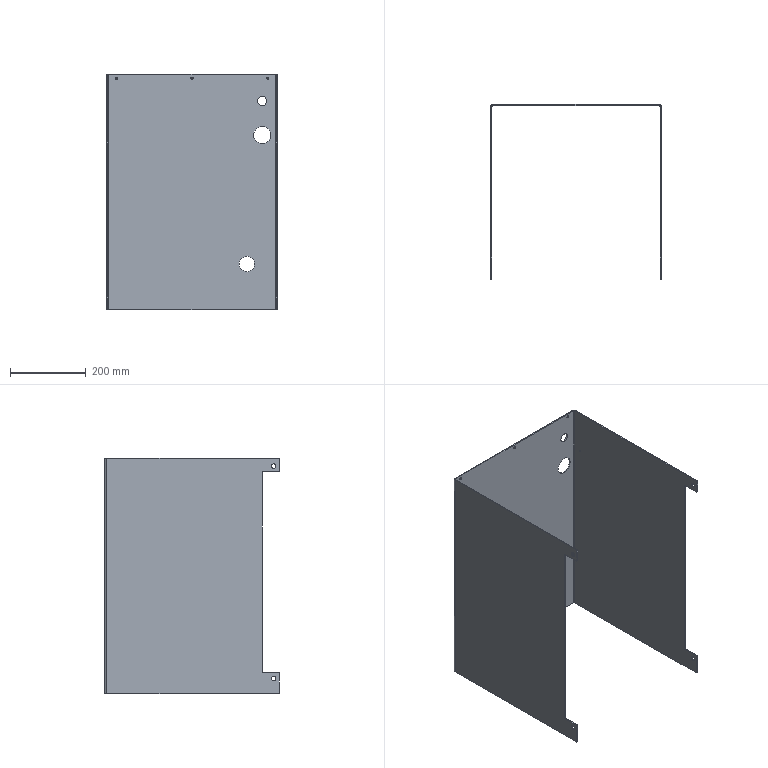Part | SolidWorks | features ICE 3, Fillet 1, FlatPattern 1, LPattern 1, SMBaseFlange 1, SheetMetal 1, SweepThread 1 | 1 solid | 83 faces | box 450 x 461 x 620 mm | volume 2378784 mm3 | cylinder 45 | plane 29 | spline 9 | commonest cylinder face diameters 5 x21 12 x10 6 x6 5.2 x2 24.2 x2 40.5 x2